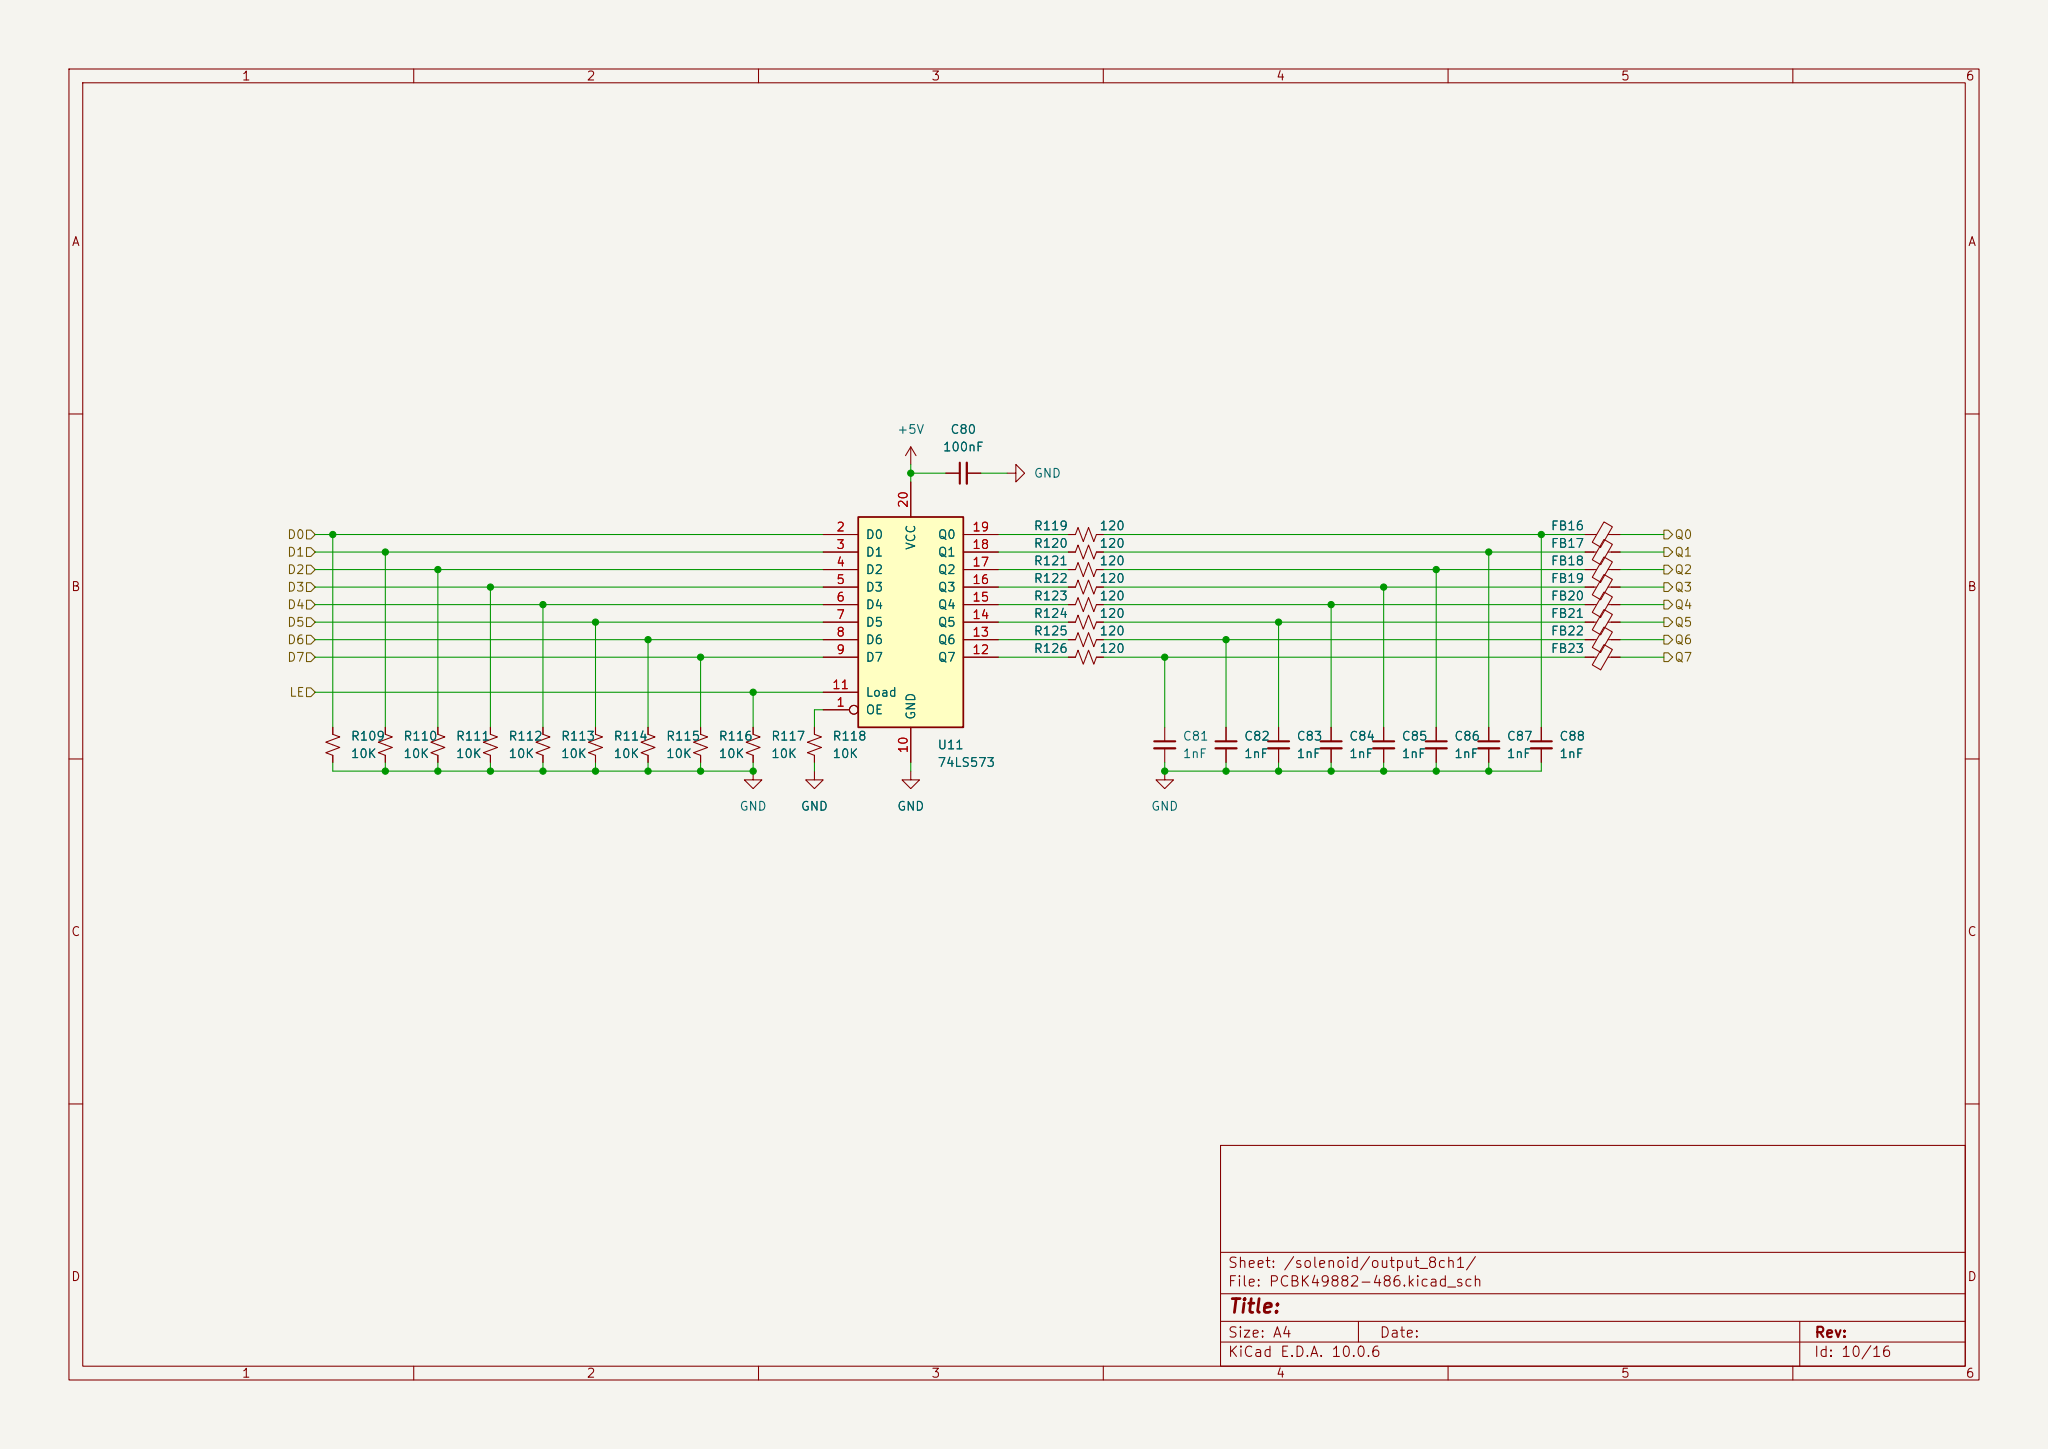Circuit board | KiCad | 536 parts | 438 nets | one sheet of the schematic
Parts on this sheet (reference | value | footprint):
C80 | 100nF | Capacitor_SMD:C_0603_1608Metric
C81
C82
C83
C84
C85
C86
C87
C88
FB16
FB17
FB18
FB19
FB20
FB21
FB22
FB23
R109
R110
R111
R112
R113
R114
R115
R116
R117
R118
R119
R120
R121
R122
R123
R124
R125
R126
U11
Nets of these parts (net: part-pin ...):
+5V: C80-1 U11-20
/core_board_b2b/PA0_C{slash}ADC12_INP0: R109-1 U11-2
/core_board_b2b/PA1_C{slash}ADC12_INP1: R110-1 U11-3
/core_board_b2b/PA3{slash}ADC12_INP15: R113-1 U11-6
/core_board_b2b/PA4{slash}ADC12_INP18: R114-1 U11-7
/core_board_b2b/PA5{slash}ADC12_INP19: R115-1 U11-8
/core_board_b2b/PA6{slash}ADC12_INP3: R116-1 U11-9
/core_board_b2b/PB1{slash}ADC12_INP5: R117-1 U11-11
/core_board_b2b/PC2_C{slash}ADC3_INP0: R111-1 U11-4
/core_board_b2b/PC3_C{slash}ADC3_INP1: R112-1 U11-5
/solenoid/OUTPUT8: FB16-2
/solenoid/OUTPUT9: FB17-2
/solenoid/OUTPUT10: FB18-2
/solenoid/OUTPUT11: FB19-2
/solenoid/OUTPUT12: FB20-2
/solenoid/OUTPUT13: FB21-2
/solenoid/OUTPUT14: FB22-2
/solenoid/OUTPUT15: FB23-2
GND: C80-2 C81-2 C82-2 C83-2 C84-2 C85-2 C86-2 C87-2 C88-2 R109-2 R110-2 R111-2 R112-2 R113-2 R114-2 R115-2 R116-2 R117-2 R118-2 U11-10
Net-(C81-Pad1): C81-1 FB23-1 R126-2
Net-(C82-Pad1): C82-1 FB22-1 R125-2
Net-(C83-Pad1): C83-1 FB21-1 R124-2
Net-(C84-Pad1): C84-1 FB20-1 R123-2
Net-(C85-Pad1): C85-1 FB19-1 R122-2
Net-(C86-Pad1): C86-1 FB18-1 R121-2
Net-(C87-Pad1): C87-1 FB17-1 R120-2
Net-(C88-Pad1): C88-1 FB16-1 R119-2
Net-(U11-OE): R118-1 U11-1
Net-(U11-Q0): R119-1 U11-19
Net-(U11-Q1): R120-1 U11-18
Net-(U11-Q2): R121-1 U11-17
Net-(U11-Q3): R122-1 U11-16
Net-(U11-Q4): R123-1 U11-15
Net-(U11-Q5): R124-1 U11-14
Net-(U11-Q6): R125-1 U11-13
Net-(U11-Q7): R126-1 U11-12